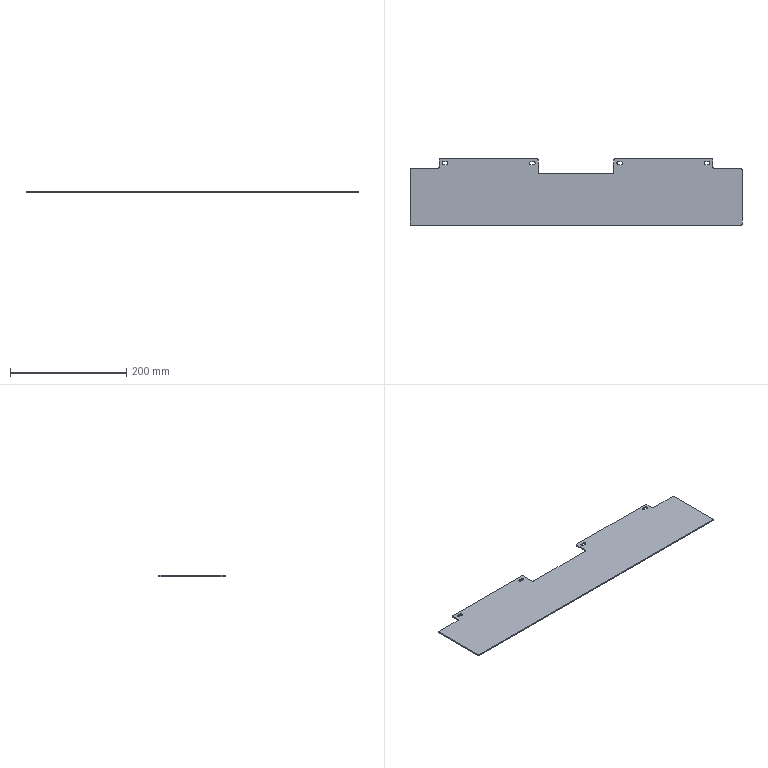Part | STEP file | 1 solid | 46 faces | box 570 x 114 x 2 mm | volume 119896 mm3 | cylinder 24 | plane 22 | commonest cylinder face diameters 4 x12 5 x12